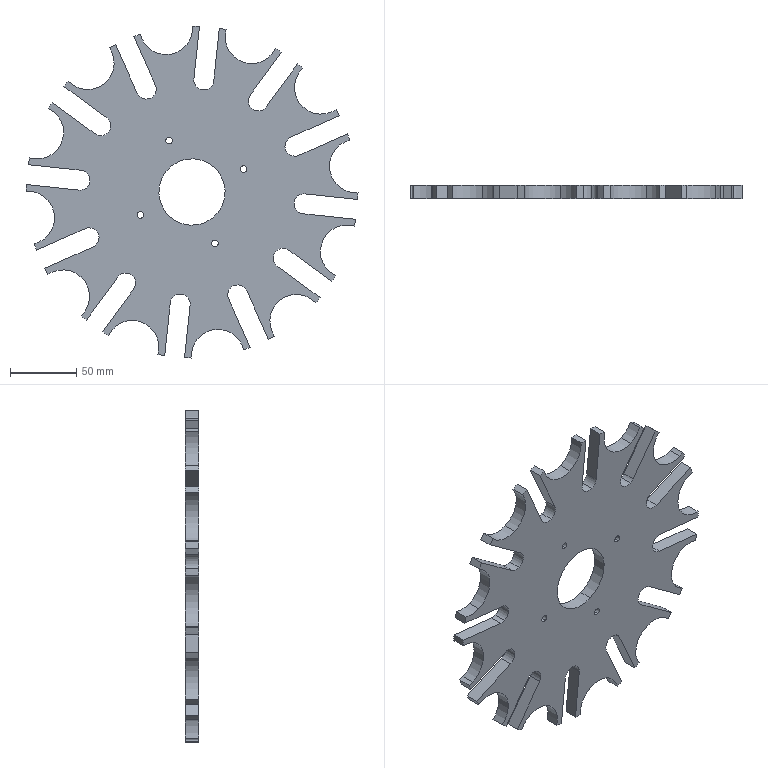Part | STEP file | M6 threaded hole 1-2 | 1 solid | 106 faces | box 249.998 x 10 x 249.998 mm | volume 314744 mm3 | cylinder 80 | plane 26 | commonest cylinder face diameters 40 x24 250 x24 15 x22 5 x8 50 x2